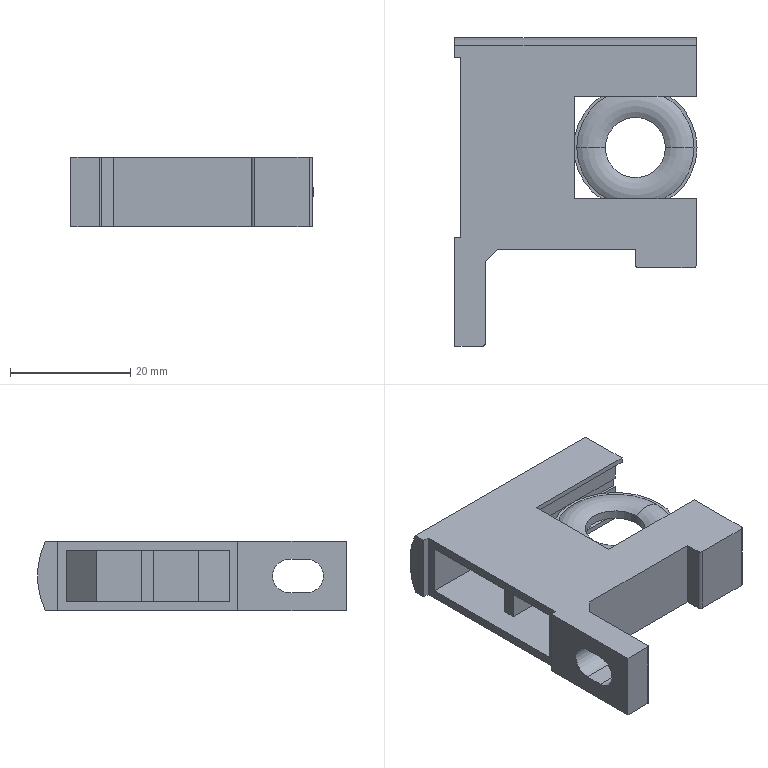Part | SolidWorks | features RefAxis 12, ICE 6, 3DProfileFeature 4, RevCut 2, Extrusion 1, Revolution 1 | 1 solid | 69 faces | box 40.25 x 51.3 x 11.5 mm | volume 9114 mm3 | plane 51 | cylinder 14 | torus 4 | commonest cylinder face diameters 4 x4 1 x2 5.5 x2 10 x2 20.5 x2 0.6 x1